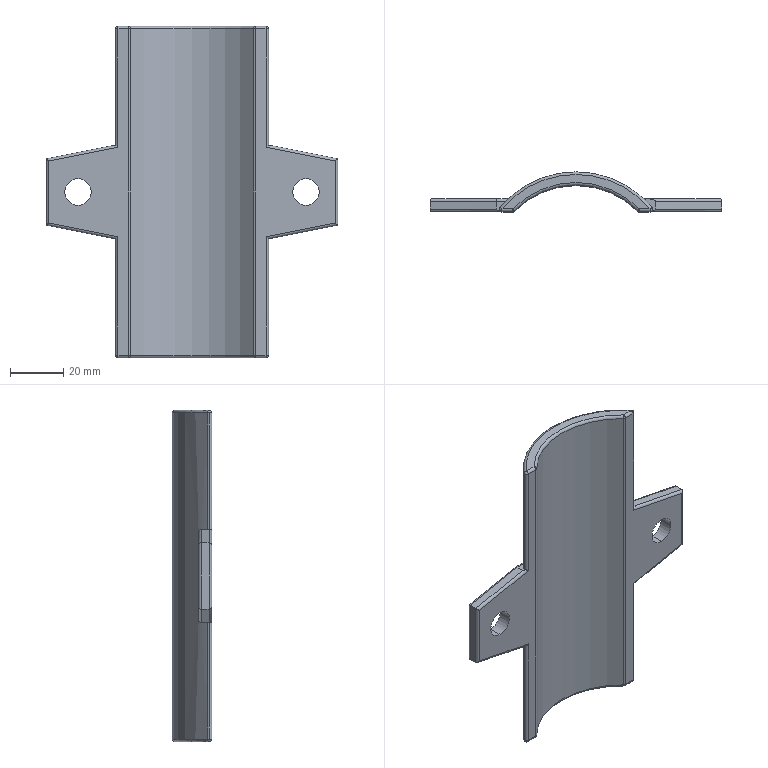Part | SolidWorks | features Chamfer 4, Fillet 2, ICE 2, ExtruThin 1, HoleWzd 1 | 1 solid | 62 faces | box 110 x 15 x 125 mm | volume 45305 mm3 | cylinder 32 | plane 16 | sphere 10 | torus 4 | commonest cylinder face diameters 2 x26 10 x4 65 x1 75 x1